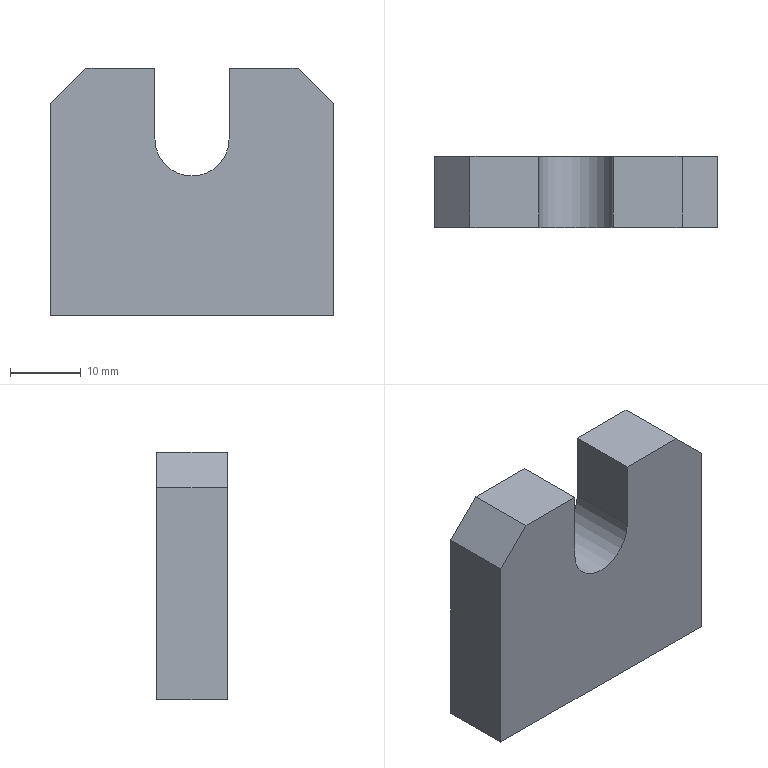Part | STEP file | PN_0038 | 1 solid | 20 faces | box 40 x 10 x 35 mm | volume 12065 mm3 | plane 11 | cylinder 5 | cone 4 | commonest cylinder face diameters 3.3 x4 10.5 x1
STEP:
#1=CARTESIAN_POINT('',(0.,0.,0.));
#2=DIRECTION('',(0.,0.,1.));
#3=DIRECTION('',(1.,0.,0.));
#4=AXIS2_PLACEMENT_3D('',#1,#2,#3);
#5=CARTESIAN_POINT('',(5.85,5.,-6.));
#6=VERTEX_POINT('',#5);
#7=CARTESIAN_POINT('',(5.85,5.,-17.5));
#8=VERTEX_POINT('',#7);
#9=CARTESIAN_POINT('',(5.85,5.,-17.5));
#10=DIRECTION('',(0.,0.,-1.));
#11=VECTOR('',#10,1.);
#12=LINE('',#9,#11);
#13=CARTESIAN_POINT('',(7.5,5.,-17.5));
#14=DIRECTION('',(0.,0.,-1.));
#15=DIRECTION('',(-1.,0.,0.));
#16=AXIS2_PLACEMENT_3D('',#13,#14,#15);
#17=CYLINDRICAL_SURFACE('',#16,1.65);
#18=CARTESIAN_POINT('',(6.283,0.));
#19=DIRECTION('',(0.,1.));
#20=VECTOR('',#19,1.);
#21=LINE('',#18,#20);
#22=(GEOMETRIC_REPRESENTATION_CONTEXT(2)PARAMETRIC_REPRESENTATION_CONTEXT()REPRESENTATION_CONTEXT('',''));
#23=DEFINITIONAL_REPRESENTATION('',(#21),#22);
#24=PCURVE('',#17,#23);
#25=CARTESIAN_POINT('',(7.5,5.,-17.5));
#26=DIRECTION('',(0.,0.,-1.));
#27=DIRECTION('',(-1.,0.,0.));
#28=AXIS2_PLACEMENT_3D('',#25,#26,#27);
#29=CYLINDRICAL_SURFACE('',#28,1.65);
#30=CARTESIAN_POINT('',(0.,0.));
#31=DIRECTION('',(0.,1.));
#32=VECTOR('',#31,1.);
#33=LINE('',#30,#32);
#34=(GEOMETRIC_REPRESENTATION_CONTEXT(2)PARAMETRIC_REPRESENTATION_CONTEXT()REPRESENTATION_CONTEXT('',''));
#35=DEFINITIONAL_REPRESENTATION('',(#33),#34);
#36=PCURVE('',#29,#35);
#37=SURFACE_CURVE('',#12,(#24,#36),.PCURVE_S1.);
#38=EDGE_CURVE('',#6,#8,#37,.T.);
#39=ORIENTED_EDGE('',*,*,#38,.T.);
#40=CARTESIAN_POINT('',(9.15,5.,-17.5));
#41=VERTEX_POINT('',#40);
#42=CARTESIAN_POINT('',(7.5,5.,-17.5));
#43=DIRECTION('',(0.,0.,-1.));
#44=DIRECTION('',(-1.,0.,0.));
#45=AXIS2_PLACEMENT_3D('',#42,#43,#44);
#46=CIRCLE('',#45,1.65);
#47=CARTESIAN_POINT('',(0.,0.));
#48=DIRECTION('',(1.,0.));
#49=VECTOR('',#48,1.);
#50=LINE('',#47,#49);
#51=(GEOMETRIC_REPRESENTATION_CONTEXT(2)PARAMETRIC_REPRESENTATION_CONTEXT()REPRESENTATION_CONTEXT('',''));
#52=DEFINITIONAL_REPRESENTATION('',(#50),#51);
#53=PCURVE('',#17,#52);
#54=CARTESIAN_POINT('',(-20.,10.,-17.5));
#55=DIRECTION('',(0.,0.,1.));
#56=DIRECTION('',(1.,0.,0.));
#57=AXIS2_PLACEMENT_3D('',#54,#55,#56);
#58=PLANE('',#57);
#59=CARTESIAN_POINT('',(25.85,-5.));
#60=CARTESIAN_POINT('',(25.85,-2.142));
#61=CARTESIAN_POINT('',(28.325,-3.571));
#62=CARTESIAN_POINT('',(30.8,-5.));
#63=CARTESIAN_POINT('',(28.325,-6.429));
#64=CARTESIAN_POINT('',(25.85,-7.858));
#65=CARTESIAN_POINT('',(25.85,-5.));
#66=(BOUNDED_CURVE()B_SPLINE_CURVE(2,(#59,#60,#61,#62,#63,#64,#65),.UNSPECIFIED.,.T.,.F.)B_SPLINE_CURVE_WITH_KNOTS((1,2,2,2,2,1),(-2.094,0.,2.094,4.189,6.283,8.378),.UNSPECIFIED.)CURVE()GEOMETRIC_REPRESENTATION_ITEM()RATIONAL_B_SPLINE_CURVE((1.,0.5,1.,0.5,1.,0.5,1.))REPRESENTATION_ITEM(''));
#67=(GEOMETRIC_REPRESENTATION_CONTEXT(2)PARAMETRIC_REPRESENTATION_CONTEXT()REPRESENTATION_CONTEXT('',''));
#68=DEFINITIONAL_REPRESENTATION('',(#66),#67);
#69=PCURVE('',#58,#68);
#70=SURFACE_CURVE('',#46,(#53,#69),.PCURVE_S1.);
#71=EDGE_CURVE('',#41,#8,#70,.T.);
#72=ORIENTED_EDGE('',*,*,#71,.F.);
#73=CARTESIAN_POINT('',(9.15,5.,-6.));
#74=VERTEX_POINT('',#73);
#75=CARTESIAN_POINT('',(9.15,5.,-17.5));
#76=DIRECTION('',(0.,0.,-1.));
#77=VECTOR('',#76,1.);
#78=LINE('',#75,#77);
#79=CARTESIAN_POINT('',(3.142,0.));
#80=DIRECTION('',(0.,1.));
#81=VECTOR('',#80,1.);
#82=LINE('',#79,#81);
#83=(GEOMETRIC_REPRESENTATION_CONTEXT(2)PARAMETRIC_REPRESENTATION_CONTEXT()REPRESENTATION_CONTEXT('',''));
#84=DEFINITIONAL_REPRESENTATION('',(#82),#83);
#85=PCURVE('',#17,#84);
#86=CARTESIAN_POINT('',(3.142,0.));
#87=DIRECTION('',(0.,1.));
#88=VECTOR('',#87,1.);
#89=LINE('',#86,#88);
#90=(GEOMETRIC_REPRESENTATION_CONTEXT(2)PARAMETRIC_REPRESENTATION_CONTEXT()REPRESENTATION_CONTEXT('',''));
#91=DEFINITIONAL_REPRESENTATION('',(#89),#90);
#92=PCURVE('',#29,#91);
#93=SURFACE_CURVE('',#78,(#85,#92),.PCURVE_S1.);
#94=EDGE_CURVE('',#74,#41,#93,.T.);
#95=ORIENTED_EDGE('',*,*,#94,.F.);
#96=CARTESIAN_POINT('',(7.5,5.,-6.));
#97=DIRECTION('',(0.,0.,-1.));
#98=DIRECTION('',(-1.,0.,0.));
#99=AXIS2_PLACEMENT_3D('',#96,#97,#98);
#100=CIRCLE('',#99,1.65);
#101=CARTESIAN_POINT('',(0.,-11.5));
#102=DIRECTION('',(1.,0.));
#103=VECTOR('',#102,1.);
#104=LINE('',#101,#103);
#105=(GEOMETRIC_REPRESENTATION_CONTEXT(2)PARAMETRIC_REPRESENTATION_CONTEXT()REPRESENTATION_CONTEXT('',''));
#106=DEFINITIONAL_REPRESENTATION('',(#104),#105);
#107=PCURVE('',#17,#106);
#108=CARTESIAN_POINT('',(7.5,5.,-6.));
#109=DIRECTION('',(0.,0.,-1.));
#110=DIRECTION('',(-1.,0.,0.));
#111=AXIS2_PLACEMENT_3D('',#108,#109,#110);
#112=CONICAL_SURFACE('',#111,1.65,1.03);
#113=CARTESIAN_POINT('',(0.,0.));
#114=DIRECTION('',(1.,0.));
#115=VECTOR('',#114,1.);
#116=LINE('',#113,#115);
#117=(GEOMETRIC_REPRESENTATION_CONTEXT(2)PARAMETRIC_REPRESENTATION_CONTEXT()REPRESENTATION_CONTEXT('',''));
#118=DEFINITIONAL_REPRESENTATION('',(#116),#117);
#119=PCURVE('',#112,#118);
#120=SURFACE_CURVE('',#100,(#107,#119),.PCURVE_S1.);
#121=EDGE_CURVE('',#74,#6,#120,.T.);
#122=ORIENTED_EDGE('',*,*,#121,.T.);
#123=EDGE_LOOP('',(#39,#72,#95,#122));
#124=FACE_BOUND('',#123,.F.);
#125=ADVANCED_FACE('',(#124),#17,.F.);
#126=ORIENTED_EDGE('',*,*,#121,.F.);
#127=CARTESIAN_POINT('',(7.5,5.,-5.009));
#128=VERTEX_POINT('',#127);
#129=CARTESIAN_POINT('',(9.15,5.,-6.));
#130=DIRECTION('',(0.8572,0.,-0.515));
#131=VECTOR('',#130,1.);
#132=LINE('',#129,#131);
#133=CARTESIAN_POINT('',(3.142,0.));
#134=DIRECTION('',(0.,1.));
#135=VECTOR('',#134,1.);
#136=LINE('',#133,#135);
#137=(GEOMETRIC_REPRESENTATION_CONTEXT(2)PARAMETRIC_REPRESENTATION_CONTEXT()REPRESENTATION_CONTEXT('',''));
#138=DEFINITIONAL_REPRESENTATION('',(#136),#137);
#139=PCURVE('',#112,#138);
#140=CARTESIAN_POINT('',(7.5,5.,-6.));
#141=DIRECTION('',(0.,0.,-1.));
#142=DIRECTION('',(-1.,0.,0.));
#143=AXIS2_PLACEMENT_3D('',#140,#141,#142);
#144=CONICAL_SURFACE('',#143,1.65,1.03);
#145=CARTESIAN_POINT('',(3.142,0.));
#146=DIRECTION('',(0.,1.));
#147=VECTOR('',#146,1.);
#148=LINE('',#145,#147);
#149=(GEOMETRIC_REPRESENTATION_CONTEXT(2)PARAMETRIC_REPRESENTATION_CONTEXT()REPRESENTATION_CONTEXT('',''));
#150=DEFINITIONAL_REPRESENTATION('',(#148),#149);
#151=PCURVE('',#144,#150);
#152=SURFACE_CURVE('',#132,(#139,#151),.PCURVE_S1.);
#153=EDGE_CURVE('',#128,#74,#152,.T.);
#154=ORIENTED_EDGE('',*,*,#153,.F.);
#155=CARTESIAN_POINT('',(5.85,5.,-6.));
#156=DIRECTION('',(-0.8572,0.,-0.515));
#157=VECTOR('',#156,1.);
#158=LINE('',#155,#157);
#159=CARTESIAN_POINT('',(6.283,0.));
#160=DIRECTION('',(0.,1.));
#161=VECTOR('',#160,1.);
#162=LINE('',#159,#161);
#163=(GEOMETRIC_REPRESENTATION_CONTEXT(2)PARAMETRIC_REPRESENTATION_CONTEXT()REPRESENTATION_CONTEXT('',''));
#164=DEFINITIONAL_REPRESENTATION('',(#162),#163);
#165=PCURVE('',#112,#164);
#166=CARTESIAN_POINT('',(0.,0.));
#167=DIRECTION('',(0.,1.));
#168=VECTOR('',#167,1.);
#169=LINE('',#166,#168);
#170=(GEOMETRIC_REPRESENTATION_CONTEXT(2)PARAMETRIC_REPRESENTATION_CONTEXT()REPRESENTATION_CONTEXT('',''));
#171=DEFINITIONAL_REPRESENTATION('',(#169),#170);
#172=PCURVE('',#144,#171);
#173=SURFACE_CURVE('',#158,(#165,#172),.PCURVE_S1.);
#174=EDGE_CURVE('',#128,#6,#173,.T.);
#175=ORIENTED_EDGE('',*,*,#174,.T.);
#176=EDGE_LOOP('',(#126,#154,#175));
#177=FACE_BOUND('',#176,.F.);
#178=ADVANCED_FACE('',(#177),#112,.F.);
#179=CARTESIAN_POINT('',(-9.15,5.,-6.));
#180=VERTEX_POINT('',#179);
#181=CARTESIAN_POINT('',(-9.15,5.,-17.5));
#182=VERTEX_POINT('',#181);
#183=CARTESIAN_POINT('',(-9.15,5.,-17.5));
#184=DIRECTION('',(0.,0.,-1.));
#185=VECTOR('',#184,1.);
#186=LINE('',#183,#185);
#187=CARTESIAN_POINT('',(-7.5,5.,-17.5));
#188=DIRECTION('',(0.,0.,-1.));
#189=DIRECTION('',(-1.,0.,0.));
#190=AXIS2_PLACEMENT_3D('',#187,#188,#189);
#191=CYLINDRICAL_SURFACE('',#190,1.65);
#192=CARTESIAN_POINT('',(6.283,0.));
#193=DIRECTION('',(0.,1.));
#194=VECTOR('',#193,1.);
#195=LINE('',#192,#194);
#196=(GEOMETRIC_REPRESENTATION_CONTEXT(2)PARAMETRIC_REPRESENTATION_CONTEXT()REPRESENTATION_CONTEXT('',''));
#197=DEFINITIONAL_REPRESENTATION('',(#195),#196);
#198=PCURVE('',#191,#197);
#199=CARTESIAN_POINT('',(-7.5,5.,-17.5));
#200=DIRECTION('',(0.,0.,-1.));
#201=DIRECTION('',(-1.,0.,0.));
#202=AXIS2_PLACEMENT_3D('',#199,#200,#201);
#203=CYLINDRICAL_SURFACE('',#202,1.65);
#204=CARTESIAN_POINT('',(0.,0.));
#205=DIRECTION('',(0.,1.));
#206=VECTOR('',#205,1.);
#207=LINE('',#204,#206);
#208=(GEOMETRIC_REPRESENTATION_CONTEXT(2)PARAMETRIC_REPRESENTATION_CONTEXT()REPRESENTATION_CONTEXT('',''));
#209=DEFINITIONAL_REPRESENTATION('',(#207),#208);
#210=PCURVE('',#203,#209);
#211=SURFACE_CURVE('',#186,(#198,#210),.PCURVE_S1.);
#212=EDGE_CURVE('',#180,#182,#211,.T.);
#213=ORIENTED_EDGE('',*,*,#212,.T.);
#214=CARTESIAN_POINT('',(-5.85,5.,-17.5));
#215=VERTEX_POINT('',#214);
#216=CARTESIAN_POINT('',(-7.5,5.,-17.5));
#217=DIRECTION('',(0.,0.,-1.));
#218=DIRECTION('',(-1.,0.,0.));
#219=AXIS2_PLACEMENT_3D('',#216,#217,#218);
#220=CIRCLE('',#219,1.65);
#221=CARTESIAN_POINT('',(0.,0.));
#222=DIRECTION('',(1.,0.));
#223=VECTOR('',#222,1.);
#224=LINE('',#221,#223);
#225=(GEOMETRIC_REPRESENTATION_CONTEXT(2)PARAMETRIC_REPRESENTATION_CONTEXT()REPRESENTATION_CONTEXT('',''));
#226=DEFINITIONAL_REPRESENTATION('',(#224),#225);
#227=PCURVE('',#191,#226);
#228=CARTESIAN_POINT('',(10.85,-5.));
#229=CARTESIAN_POINT('',(10.85,-2.142));
#230=CARTESIAN_POINT('',(13.325,-3.571));
#231=CARTESIAN_POINT('',(15.8,-5.));
#232=CARTESIAN_POINT('',(13.325,-6.429));
#233=CARTESIAN_POINT('',(10.85,-7.858));
#234=CARTESIAN_POINT('',(10.85,-5.));
#235=(BOUNDED_CURVE()B_SPLINE_CURVE(2,(#228,#229,#230,#231,#232,#233,#234),.UNSPECIFIED.,.T.,.F.)B_SPLINE_CURVE_WITH_KNOTS((1,2,2,2,2,1),(-2.094,0.,2.094,4.189,6.283,8.378),.UNSPECIFIED.)CURVE()GEOMETRIC_REPRESENTATION_ITEM()RATIONAL_B_SPLINE_CURVE((1.,0.5,1.,0.5,1.,0.5,1.))REPRESENTATION_ITEM(''));
#236=(GEOMETRIC_REPRESENTATION_CONTEXT(2)PARAMETRIC_REPRESENTATION_CONTEXT()REPRESENTATION_CONTEXT('',''));
#237=DEFINITIONAL_REPRESENTATION('',(#235),#236);
#238=PCURVE('',#58,#237);
#239=SURFACE_CURVE('',#220,(#227,#238),.PCURVE_S1.);
#240=EDGE_CURVE('',#215,#182,#239,.T.);
#241=ORIENTED_EDGE('',*,*,#240,.F.);
#242=CARTESIAN_POINT('',(-5.85,5.,-6.));
#243=VERTEX_POINT('',#242);
#244=CARTESIAN_POINT('',(-5.85,5.,-17.5));
#245=DIRECTION('',(0.,0.,-1.));
#246=VECTOR('',#245,1.);
#247=LINE('',#244,#246);
#248=CARTESIAN_POINT('',(3.142,0.));
#249=DIRECTION('',(0.,1.));
#250=VECTOR('',#249,1.);
#251=LINE('',#248,#250);
#252=(GEOMETRIC_REPRESENTATION_CONTEXT(2)PARAMETRIC_REPRESENTATION_CONTEXT()REPRESENTATION_CONTEXT('',''));
#253=DEFINITIONAL_REPRESENTATION('',(#251),#252);
#254=PCURVE('',#191,#253);
#255=CARTESIAN_POINT('',(3.142,0.));
#256=DIRECTION('',(0.,1.));
#257=VECTOR('',#256,1.);
#258=LINE('',#255,#257);
#259=(GEOMETRIC_REPRESENTATION_CONTEXT(2)PARAMETRIC_REPRESENTATION_CONTEXT()REPRESENTATION_CONTEXT('',''));
#260=DEFINITIONAL_REPRESENTATION('',(#258),#259);
#261=PCURVE('',#203,#260);
#262=SURFACE_CURVE('',#247,(#254,#261),.PCURVE_S1.);
#263=EDGE_CURVE('',#243,#215,#262,.T.);
#264=ORIENTED_EDGE('',*,*,#263,.F.);
#265=CARTESIAN_POINT('',(-7.5,5.,-6.));
#266=DIRECTION('',(0.,0.,-1.));
#267=DIRECTION('',(-1.,0.,0.));
#268=AXIS2_PLACEMENT_3D('',#265,#266,#267);
#269=CIRCLE('',#268,1.65);
#270=CARTESIAN_POINT('',(0.,-11.5));
#271=DIRECTION('',(1.,0.));
#272=VECTOR('',#271,1.);
#273=LINE('',#270,#272);
#274=(GEOMETRIC_REPRESENTATION_CONTEXT(2)PARAMETRIC_REPRESENTATION_CONTEXT()REPRESENTATION_CONTEXT('',''));
#275=DEFINITIONAL_REPRESENTATION('',(#273),#274);
#276=PCURVE('',#191,#275);
#277=CARTESIAN_POINT('',(-7.5,5.,-6.));
#278=DIRECTION('',(0.,0.,-1.));
#279=DIRECTION('',(-1.,0.,0.));
#280=AXIS2_PLACEMENT_3D('',#277,#278,#279);
#281=CONICAL_SURFACE('',#280,1.65,1.03);
#282=CARTESIAN_POINT('',(0.,0.));
#283=DIRECTION('',(1.,0.));
#284=VECTOR('',#283,1.);
#285=LINE('',#282,#284);
#286=(GEOMETRIC_REPRESENTATION_CONTEXT(2)PARAMETRIC_REPRESENTATION_CONTEXT()REPRESENTATION_CONTEXT('',''));
#287=DEFINITIONAL_REPRESENTATION('',(#285),#286);
#288=PCURVE('',#281,#287);
#289=SURFACE_CURVE('',#269,(#276,#288),.PCURVE_S1.);
#290=EDGE_CURVE('',#243,#180,#289,.T.);
#291=ORIENTED_EDGE('',*,*,#290,.T.);
#292=EDGE_LOOP('',(#213,#241,#264,#291));
#293=FACE_BOUND('',#292,.F.);
#294=ADVANCED_FACE('',(#293),#191,.F.);
#295=ORIENTED_EDGE('',*,*,#290,.F.);
#296=CARTESIAN_POINT('',(-7.5,5.,-5.009));
#297=VERTEX_POINT('',#296);
#298=CARTESIAN_POINT('',(-5.85,5.,-6.));
#299=DIRECTION('',(0.8572,0.,-0.515));
#300=VECTOR('',#299,1.);
#301=LINE('',#298,#300);
#302=CARTESIAN_POINT('',(3.142,0.));
#303=DIRECTION('',(0.,1.));
#304=VECTOR('',#303,1.);
#305=LINE('',#302,#304);
#306=(GEOMETRIC_REPRESENTATION_CONTEXT(2)PARAMETRIC_REPRESENTATION_CONTEXT()REPRESENTATION_CONTEXT('',''));
#307=DEFINITIONAL_REPRESENTATION('',(#305),#306);
#308=PCURVE('',#281,#307);
#309=CARTESIAN_POINT('',(-7.5,5.,-6.));
#310=DIRECTION('',(0.,0.,-1.));
#311=DIRECTION('',(-1.,0.,0.));
#312=AXIS2_PLACEMENT_3D('',#309,#310,#311);
#313=CONICAL_SURFACE('',#312,1.65,1.03);
#314=CARTESIAN_POINT('',(3.142,0.));
#315=DIRECTION('',(0.,1.));
#316=VECTOR('',#315,1.);
#317=LINE('',#314,#316);
#318=(GEOMETRIC_REPRESENTATION_CONTEXT(2)PARAMETRIC_REPRESENTATION_CONTEXT()REPRESENTATION_CONTEXT('',''));
#319=DEFINITIONAL_REPRESENTATION('',(#317),#318);
#320=PCURVE('',#313,#319);
#321=SURFACE_CURVE('',#301,(#308,#320),.PCURVE_S1.);
#322=EDGE_CURVE('',#297,#243,#321,.T.);
#323=ORIENTED_EDGE('',*,*,#322,.F.);
#324=CARTESIAN_POINT('',(-9.15,5.,-6.));
#325=DIRECTION('',(-0.8572,0.,-0.515));
#326=VECTOR('',#325,1.);
#327=LINE('',#324,#326);
#328=CARTESIAN_POINT('',(6.283,0.));
#329=DIRECTION('',(0.,1.));
#330=VECTOR('',#329,1.);
#331=LINE('',#328,#330);
#332=(GEOMETRIC_REPRESENTATION_CONTEXT(2)PARAMETRIC_REPRESENTATION_CONTEXT()REPRESENTATION_CONTEXT('',''));
#333=DEFINITIONAL_REPRESENTATION('',(#331),#332);
#334=PCURVE('',#281,#333);
#335=CARTESIAN_POINT('',(0.,0.));
#336=DIRECTION('',(0.,1.));
#337=VECTOR('',#336,1.);
#338=LINE('',#335,#337);
#339=(GEOMETRIC_REPRESENTATION_CONTEXT(2)PARAMETRIC_REPRESENTATION_CONTEXT()REPRESENTATION_CONTEXT('',''));
#340=DEFINITIONAL_REPRESENTATION('',(#338),#339);
#341=PCURVE('',#313,#340);
#342=SURFACE_CURVE('',#327,(#334,#341),.PCURVE_S1.);
#343=EDGE_CURVE('',#297,#180,#342,.T.);
#344=ORIENTED_EDGE('',*,*,#343,.T.);
#345=EDGE_LOOP('',(#295,#323,#344));
#346=FACE_BOUND('',#345,.F.);
#347=ADVANCED_FACE('',(#346),#281,.F.);
#348=CARTESIAN_POINT('',(5.25,10.,17.5));
#349=VERTEX_POINT('',#348);
#350=CARTESIAN_POINT('',(15.,10.,17.5));
#351=VERTEX_POINT('',#350);
#352=CARTESIAN_POINT('',(-20.,10.,17.5));
#353=DIRECTION('',(1.,0.,0.));
#354=VECTOR('',#353,1.);
#355=LINE('',#352,#354);
#356=CARTESIAN_POINT('',(-20.,10.,17.5));
#357=DIRECTION('',(0.,0.,-1.));
#358=DIRECTION('',(-1.,0.,0.));
#359=AXIS2_PLACEMENT_3D('',#356,#357,#358);
#360=PLANE('',#359);
#361=CARTESIAN_POINT('',(0.,0.));
#362=DIRECTION('',(-1.,0.));
#363=VECTOR('',#362,1.);
#364=LINE('',#361,#363);
#365=(GEOMETRIC_REPRESENTATION_CONTEXT(2)PARAMETRIC_REPRESENTATION_CONTEXT()REPRESENTATION_CONTEXT('',''));
#366=DEFINITIONAL_REPRESENTATION('',(#364),#365);
#367=PCURVE('',#360,#366);
#368=CARTESIAN_POINT('',(0.,10.,0.));
#369=DIRECTION('',(0.,1.,0.));
#370=DIRECTION('',(0.,0.,1.));
#371=AXIS2_PLACEMENT_3D('',#368,#369,#370);
#372=PLANE('',#371);
#373=CARTESIAN_POINT('',(17.5,-20.));
#374=DIRECTION('',(0.,1.));
#375=VECTOR('',#374,1.);
#376=LINE('',#373,#375);
#377=(GEOMETRIC_REPRESENTATION_CONTEXT(2)PARAMETRIC_REPRESENTATION_CONTEXT()REPRESENTATION_CONTEXT('',''));
#378=DEFINITIONAL_REPRESENTATION('',(#376),#377);
#379=PCURVE('',#372,#378);
#380=SURFACE_CURVE('',#355,(#367,#379),.PCURVE_S1.);
#381=EDGE_CURVE('',#349,#351,#380,.T.);
#382=ORIENTED_EDGE('',*,*,#381,.F.);
#383=CARTESIAN_POINT('',(5.25,0.,17.5));
#384=VERTEX_POINT('',#383);
#385=CARTESIAN_POINT('',(5.25,0.,17.5));
#386=DIRECTION('',(0.,1.,0.));
#387=VECTOR('',#386,1.);
#388=LINE('',#385,#387);
#389=CARTESIAN_POINT('',(-25.25,-10.));
#390=DIRECTION('',(0.,1.));
#391=VECTOR('',#390,1.);
#392=LINE('',#389,#391);
#393=(GEOMETRIC_REPRESENTATION_CONTEXT(2)PARAMETRIC_REPRESENTATION_CONTEXT()REPRESENTATION_CONTEXT('',''));
#394=DEFINITIONAL_REPRESENTATION('',(#392),#393);
#395=PCURVE('',#360,#394);
#396=CARTESIAN_POINT('',(5.25,0.,7.5));
#397=DIRECTION('',(1.,0.,0.));
#398=DIRECTION('',(0.,0.,-1.));
#399=AXIS2_PLACEMENT_3D('',#396,#397,#398);
#400=PLANE('',#399);
#401=CARTESIAN_POINT('',(-10.,0.));
#402=DIRECTION('',(0.,1.));
#403=VECTOR('',#402,1.);
#404=LINE('',#401,#403);
#405=(GEOMETRIC_REPRESENTATION_CONTEXT(2)PARAMETRIC_REPRESENTATION_CONTEXT()REPRESENTATION_CONTEXT('',''));
#406=DEFINITIONAL_REPRESENTATION('',(#404),#405);
#407=PCURVE('',#400,#406);
#408=SURFACE_CURVE('',#388,(#395,#407),.PCURVE_S1.);
#409=EDGE_CURVE('',#384,#349,#408,.T.);
#410=ORIENTED_EDGE('',*,*,#409,.F.);
#411=CARTESIAN_POINT('',(15.,0.,17.5));
#412=VERTEX_POINT('',#411);
#413=CARTESIAN_POINT('',(-20.,0.,17.5));
#414=DIRECTION('',(1.,0.,0.));
#415=VECTOR('',#414,1.);
#416=LINE('',#413,#415);
#417=CARTESIAN_POINT('',(0.,-10.));
#418=DIRECTION('',(-1.,0.));
#419=VECTOR('',#418,1.);
#420=LINE('',#417,#419);
#421=(GEOMETRIC_REPRESENTATION_CONTEXT(2)PARAMETRIC_REPRESENTATION_CONTEXT()REPRESENTATION_CONTEXT('',''));
#422=DEFINITIONAL_REPRESENTATION('',(#420),#421);
#423=PCURVE('',#360,#422);
#424=CARTESIAN_POINT('',(0.,0.,0.));
#425=DIRECTION('',(0.,1.,0.));
#426=DIRECTION('',(0.,0.,1.));
#427=AXIS2_PLACEMENT_3D('',#424,#425,#426);
#428=PLANE('',#427);
#429=CARTESIAN_POINT('',(17.5,-20.));
#430=DIRECTION('',(0.,1.));
#431=VECTOR('',#430,1.);
#432=LINE('',#429,#431);
#433=(GEOMETRIC_REPRESENTATION_CONTEXT(2)PARAMETRIC_REPRESENTATION_CONTEXT()REPRESENTATION_CONTEXT('',''));
#434=DEFINITIONAL_REPRESENTATION('',(#432),#433);
#435=PCURVE('',#428,#434);
#436=SURFACE_CURVE('',#416,(#423,#435),.PCURVE_S1.);
#437=EDGE_CURVE('',#384,#412,#436,.T.);
#438=ORIENTED_EDGE('',*,*,#437,.T.);
#439=CARTESIAN_POINT('',(15.,10.,17.5));
#440=DIRECTION('',(0.,1.,0.));
#441=VECTOR('',#440,1.);
#442=LINE('',#439,#441);
#443=CARTESIAN_POINT('',(-35.,0.));
#444=DIRECTION('',(0.,1.));
#445=VECTOR('',#444,1.);
#446=LINE('',#443,#445);
#447=(GEOMETRIC_REPRESENTATION_CONTEXT(2)PARAMETRIC_REPRESENTATION_CONTEXT()REPRESENTATION_CONTEXT('',''));
#448=DEFINITIONAL_REPRESENTATION('',(#446),#447);
#449=PCURVE('',#360,#448);
#450=CARTESIAN_POINT('',(20.,10.,12.5));
#451=DIRECTION('',(-0.7071,0.,-0.7071));
#452=DIRECTION('',(0.,-1.,0.));
#453=AXIS2_PLACEMENT_3D('',#450,#451,#452);
#454=PLANE('',#453);
#455=CARTESIAN_POINT('',(0.,7.071));
#456=DIRECTION('',(-1.,0.));
#457=VECTOR('',#456,1.);
#458=LINE('',#455,#457);
#459=(GEOMETRIC_REPRESENTATION_CONTEXT(2)PARAMETRIC_REPRESENTATION_CONTEXT()REPRESENTATION_CONTEXT('',''));
#460=DEFINITIONAL_REPRESENTATION('',(#458),#459);
#461=PCURVE('',#454,#460);
#462=SURFACE_CURVE('',#442,(#449,#461),.PCURVE_S1.);
#463=EDGE_CURVE('',#412,#351,#462,.T.);
#464=ORIENTED_EDGE('',*,*,#463,.T.);
#465=EDGE_LOOP('',(#382,#410,#438,#464));
#466=FACE_BOUND('',#465,.T.);
#467=ADVANCED_FACE('',(#466),#360,.F.);
#468=CARTESIAN_POINT('',(20.,10.,12.5));
#469=VERTEX_POINT('',#468);
#470=CARTESIAN_POINT('',(20.,10.,-17.5));
#471=VERTEX_POINT('',#470);
#472=CARTESIAN_POINT('',(20.,10.,-17.5));
#473=DIRECTION('',(0.,0.,-1.));
#474=VECTOR('',#473,1.);
#475=LINE('',#472,#474);
#476=CARTESIAN_POINT('',(20.,10.,-17.5));
#477=DIRECTION('',(-1.,0.,0.));
#478=DIRECTION('',(0.,0.,1.));
#479=AXIS2_PLACEMENT_3D('',#476,#477,#478);
#480=PLANE('',#479);
#481=CARTESIAN_POINT('',(0.,0.));
#482=DIRECTION('',(-1.,0.));
#483=VECTOR('',#482,1.);
#484=LINE('',#481,#483);
#485=(GEOMETRIC_REPRESENTATION_CONTEXT(2)PARAMETRIC_REPRESENTATION_CONTEXT()REPRESENTATION_CONTEXT('',''));
#486=DEFINITIONAL_REPRESENTATION('',(#484),#485);
#487=PCURVE('',#480,#486);
#488=CARTESIAN_POINT('',(-17.5,20.));
#489=DIRECTION('',(-1.,0.));
#490=VECTOR('',#489,1.);
#491=LINE('',#488,#490);
#492=(GEOMETRIC_REPRESENTATION_CONTEXT(2)PARAMETRIC_REPRESENTATION_CONTEXT()REPRESENTATION_CONTEXT('',''));
#493=DEFINITIONAL_REPRESENTATION('',(#491),#492);
#494=PCURVE('',#372,#493);
#495=SURFACE_CURVE('',#475,(#487,#494),.PCURVE_S1.);
#496=EDGE_CURVE('',#469,#471,#495,.T.);
#497=ORIENTED_EDGE('',*,*,#496,.F.);
#498=CARTESIAN_POINT('',(20.,0.,12.5));
#499=VERTEX_POINT('',#498);
#500=CARTESIAN_POINT('',(20.,10.,12.5));
#501=DIRECTION('',(0.,-1.,0.));
#502=VECTOR('',#501,1.);
#503=LINE('',#500,#502);
#504=CARTESIAN_POINT('',(30.,0.));
#505=DIRECTION('',(0.,-1.));
#506=VECTOR('',#505,1.);
#507=LINE('',#504,#506);
#508=(GEOMETRIC_REPRESENTATION_CONTEXT(2)PARAMETRIC_REPRESENTATION_CONTEXT()REPRESENTATION_CONTEXT('',''));
#509=DEFINITIONAL_REPRESENTATION('',(#507),#508);
#510=PCURVE('',#480,#509);
#511=CARTESIAN_POINT('',(0.,0.));
#512=DIRECTION('',(1.,0.));
#513=VECTOR('',#512,1.);
#514=LINE('',#511,#513);
#515=(GEOMETRIC_REPRESENTATION_CONTEXT(2)PARAMETRIC_REPRESENTATION_CONTEXT()REPRESENTATION_CONTEXT('',''));
#516=DEFINITIONAL_REPRESENTATION('',(#514),#515);
#517=PCURVE('',#454,#516);
#518=SURFACE_CURVE('',#503,(#510,#517),.PCURVE_S1.);
#519=EDGE_CURVE('',#469,#499,#518,.T.);
#520=ORIENTED_EDGE('',*,*,#519,.T.);
#521=CARTESIAN_POINT('',(20.,0.,-17.5));
#522=VERTEX_POINT('',#521);
#523=CARTESIAN_POINT('',(20.,0.,-17.5));
#524=DIRECTION('',(0.,0.,-1.));
#525=VECTOR('',#524,1.);
#526=LINE('',#523,#525);
#527=CARTESIAN_POINT('',(0.,-10.));
#528=DIRECTION('',(-1.,0.));
#529=VECTOR('',#528,1.);
#530=LINE('',#527,#529);
#531=(GEOMETRIC_REPRESENTATION_CONTEXT(2)PARAMETRIC_REPRESENTATION_CONTEXT()REPRESENTATION_CONTEXT('',''));
#532=DEFINITIONAL_REPRESENTATION('',(#530),#531);
#533=PCURVE('',#480,#532);
#534=CARTESIAN_POINT('',(-17.5,20.));
#535=DIRECTION('',(-1.,0.));
#536=VECTOR('',#535,1.);
#537=LINE('',#534,#536);
#538=(GEOMETRIC_REPRESENTATION_CONTEXT(2)PARAMETRIC_REPRESENTATION_CONTEXT()REPRESENTATION_CONTEXT('',''));
#539=DEFINITIONAL_REPRESENTATION('',(#537),#538);
#540=PCURVE('',#428,#539);
#541=SURFACE_CURVE('',#526,(#533,#540),.PCURVE_S1.);
#542=EDGE_CURVE('',#499,#522,#541,.T.);
#543=ORIENTED_EDGE('',*,*,#542,.T.);
#544=CARTESIAN_POINT('',(20.,10.,-17.5));
#545=DIRECTION('',(0.,-1.,0.));
#546=VECTOR('',#545,1.);
#547=LINE('',#544,#546);
#548=CARTESIAN_POINT('',(0.,0.));
#549=DIRECTION('',(0.,-1.));
#550=VECTOR('',#549,1.);
#551=LINE('',#548,#550);
#552=(GEOMETRIC_REPRESENTATION_CONTEXT(2)PARAMETRIC_REPRESENTATION_CONTEXT()REPRESENTATION_CONTEXT('',''));
#553=DEFINITIONAL_REPRESENTATION('',(#551),#552);
#554=PCURVE('',#480,#553);
#555=CARTESIAN_POINT('',(40.,0.));
#556=DIRECTION('',(0.,-1.));
#557=VECTOR('',#556,1.);
#558=LINE('',#555,#557);
#559=(GEOMETRIC_REPRESENTATION_CONTEXT(2)PARAMETRIC_REPRESENTATION_CONTEXT()REPRESENTATION_CONTEXT('',''));
#560=DEFINITIONAL_REPRESENTATION('',(#558),#559);
#561=PCURVE('',#58,#560);
#562=SURFACE_CURVE('',#547,(#554,#561),.PCURVE_S1.);
#563=EDGE_CURVE('',#471,#522,#562,.T.);
#564=ORIENTED_EDGE('',*,*,#563,.F.);
#565=EDGE_LOOP('',(#497,#520,#543,#564));
#566=FACE_BOUND('',#565,.T.);
#567=ADVANCED_FACE('',(#566),#480,.F.);
#568=CARTESIAN_POINT('',(7.5,5.,-17.5));
#569=DIRECTION('',(0.,0.,-1.));
#570=DIRECTION('',(-1.,0.,0.));
#571=AXIS2_PLACEMENT_3D('',#568,#569,#570);
#572=CIRCLE('',#571,1.65);
#573=CARTESIAN_POINT('',(25.85,-5.));
#574=CARTESIAN_POINT('',(25.85,-2.142));
#575=CARTESIAN_POINT('',(28.325,-3.571));
#576=CARTESIAN_POINT('',(30.8,-5.));
#577=CARTESIAN_POINT('',(28.325,-6.429));
#578=CARTESIAN_POINT('',(25.85,-7.858));
#579=CARTESIAN_POINT('',(25.85,-5.));
#580=(BOUNDED_CURVE()B_SPLINE_CURVE(2,(#573,#574,#575,#576,#577,#578,#579),.UNSPECIFIED.,.T.,.F.)B_SPLINE_CURVE_WITH_KNOTS((1,2,2,2,2,1),(-2.094,0.,2.094,4.189,6.283,8.378),.UNSPECIFIED.)CURVE()GEOMETRIC_REPRESENTATION_ITEM()RATIONAL_B_SPLINE_CURVE((1.,0.5,1.,0.5,1.,0.5,1.))REPRESENTATION_ITEM(''));
#581=(GEOMETRIC_REPRESENTATION_CONTEXT(2)PARAMETRIC_REPRESENTATION_CONTEXT()REPRESENTATION_CONTEXT('',''));
#582=DEFINITIONAL_REPRESENTATION('',(#580),#581);
#583=PCURVE('',#58,#582);
#584=CARTESIAN_POINT('',(0.,0.));
#585=DIRECTION('',(1.,0.));
#586=VECTOR('',#585,1.);
#587=LINE('',#584,#586);
#588=(GEOMETRIC_REPRESENTATION_CONTEXT(2)PARAMETRIC_REPRESENTATION_CONTEXT()REPRESENTATION_CONTEXT('',''));
#589=DEFINITIONAL_REPRESENTATION('',(#587),#588);
#590=PCURVE('',#29,#589);
#591=SURFACE_CURVE('',#572,(#583,#590),.PCURVE_S1.);
#592=EDGE_CURVE('',#8,#41,#591,.T.);
#593=ORIENTED_EDGE('',*,*,#592,.F.);
#594=ORIENTED_EDGE('',*,*,#71,.F.);
#595=EDGE_LOOP('',(#593,#594));
#596=FACE_BOUND('',#595,.T.);
#597=CARTESIAN_POINT('',(-7.5,5.,-17.5));
#598=DIRECTION('',(0.,0.,-1.));
#599=DIRECTION('',(-1.,0.,0.));
#600=AXIS2_PLACEMENT_3D('',#597,#598,#599);
#601=CIRCLE('',#600,1.65);
#602=CARTESIAN_POINT('',(10.85,-5.));
#603=CARTESIAN_POINT('',(10.85,-2.142));
#604=CARTESIAN_POINT('',(13.325,-3.571));
#605=CARTESIAN_POINT('',(15.8,-5.));
#606=CARTESIAN_POINT('',(13.325,-6.429));
#607=CARTESIAN_POINT('',(10.85,-7.858));
#608=CARTESIAN_POINT('',(10.85,-5.));
#609=(BOUNDED_CURVE()B_SPLINE_CURVE(2,(#602,#603,#604,#605,#606,#607,#608),.UNSPECIFIED.,.T.,.F.)B_SPLINE_CURVE_WITH_KNOTS((1,2,2,2,2,1),(-2.094,0.,2.094,4.189,6.283,8.378),.UNSPECIFIED.)CURVE()GEOMETRIC_REPRESENTATION_ITEM()RATIONAL_B_SPLINE_CURVE((1.,0.5,1.,0.5,1.,0.5,1.))REPRESENTATION_ITEM(''));
#610=(GEOMETRIC_REPRESENTATION_CONTEXT(2)PARAMETRIC_REPRESENTATION_CONTEXT()REPRESENTATION_CONTEXT('',''));
#611=DEFINITIONAL_REPRESENTATION('',(#609),#610);
#612=PCURVE('',#58,#611);
#613=CARTESIAN_POINT('',(0.,0.));
#614=DIRECTION('',(1.,0.));
#615=VECTOR('',#614,1.);
#616=LINE('',#613,#615);
#617=(GEOMETRIC_REPRESENTATION_CONTEXT(2)PARAMETRIC_REPRESENTATION_CONTEXT()REPRESENTATION_CONTEXT('',''));
#618=DEFINITIONAL_REPRESENTATION('',(#616),#617);
#619=PCURVE('',#203,#618);
#620=SURFACE_CURVE('',#601,(#612,#619),.PCURVE_S1.);
#621=EDGE_CURVE('',#182,#215,#620,.T.);
#622=ORIENTED_EDGE('',*,*,#621,.F.);
#623=ORIENTED_EDGE('',*,*,#240,.F.);
#624=EDGE_LOOP('',(#622,#623));
#625=FACE_BOUND('',#624,.T.);
#626=CARTESIAN_POINT('',(-20.,0.,-17.5));
#627=VERTEX_POINT('',#626);
#628=CARTESIAN_POINT('',(-20.,0.,-17.5));
#629=DIRECTION('',(-1.,0.,0.));
#630=VECTOR('',#629,1.);
#631=LINE('',#628,#630);
#632=CARTESIAN_POINT('',(0.,-10.));
#633=DIRECTION('',(-1.,0.));
#634=VECTOR('',#633,1.);
#635=LINE('',#632,#634);
#636=(GEOMETRIC_REPRESENTATION_CONTEXT(2)PARAMETRIC_REPRESENTATION_CONTEXT()REPRESENTATION_CONTEXT('',''));
#637=DEFINITIONAL_REPRESENTATION('',(#635),#636);
#638=PCURVE('',#58,#637);
#639=CARTESIAN_POINT('',(-17.5,-20.));
#640=DIRECTION('',(0.,-1.));
#641=VECTOR('',#640,1.);
#642=LINE('',#639,#641);
#643=(GEOMETRIC_REPRESENTATION_CONTEXT(2)PARAMETRIC_REPRESENTATION_CONTEXT()REPRESENTATION_CONTEXT('',''));
#644=DEFINITIONAL_REPRESENTATION('',(#642),#643);
#645=PCURVE('',#428,#644);
#646=SURFACE_CURVE('',#631,(#638,#645),.PCURVE_S1.);
#647=EDGE_CURVE('',#522,#627,#646,.T.);
#648=ORIENTED_EDGE('',*,*,#647,.T.);
#649=CARTESIAN_POINT('',(-20.,10.,-17.5));
#650=VERTEX_POINT('',#649);
#651=CARTESIAN_POINT('',(-20.,10.,-17.5));
#652=DIRECTION('',(0.,-1.,0.));
#653=VECTOR('',#652,1.);
#654=LINE('',#651,#653);
#655=CARTESIAN_POINT('',(0.,0.));
#656=DIRECTION('',(0.,-1.));
#657=VECTOR('',#656,1.);
#658=LINE('',#655,#657);
#659=(GEOMETRIC_REPRESENTATION_CONTEXT(2)PARAMETRIC_REPRESENTATION_CONTEXT()REPRESENTATION_CONTEXT('',''));
#660=DEFINITIONAL_REPRESENTATION('',(#658),#659);
#661=PCURVE('',#58,#660);
#662=CARTESIAN_POINT('',(-20.,10.,-17.5));
#663=DIRECTION('',(1.,0.,0.));
#664=DIRECTION('',(0.,0.,-1.));
#665=AXIS2_PLACEMENT_3D('',#662,#663,#664);
#666=PLANE('',#665);
#667=CARTESIAN_POINT('',(0.,0.));
#668=DIRECTION('',(0.,-1.));
#669=VECTOR('',#668,1.);
#670=LINE('',#667,#669);
#671=(GEOMETRIC_REPRESENTATION_CONTEXT(2)PARAMETRIC_REPRESENTATION_CONTEXT()REPRESENTATION_CONTEXT('',''));
#672=DEFINITIONAL_REPRESENTATION('',(#670),#671);
#673=PCURVE('',#666,#672);
#674=SURFACE_CURVE('',#654,(#661,#673),.PCURVE_S1.);
#675=EDGE_CURVE('',#650,#627,#674,.T.);
#676=ORIENTED_EDGE('',*,*,#675,.F.);
#677=CARTESIAN_POINT('',(-20.,10.,-17.5));
#678=DIRECTION('',(-1.,0.,0.));
#679=VECTOR('',#678,1.);
#680=LINE('',#677,#679);
#681=CARTESIAN_POINT('',(0.,0.));
#682=DIRECTION('',(-1.,0.));
#683=VECTOR('',#682,1.);
#684=LINE('',#681,#683);
#685=(GEOMETRIC_REPRESENTATION_CONTEXT(2)PARAMETRIC_REPRESENTATION_CONTEXT()REPRESENTATION_CONTEXT('',''));
#686=DEFINITIONAL_REPRESENTATION('',(#684),#685);
#687=PCURVE('',#58,#686);
#688=CARTESIAN_POINT('',(-17.5,-20.));
#689=DIRECTION('',(0.,-1.));
#690=VECTOR('',#689,1.);
#691=LINE('',#688,#690);
#692=(GEOMETRIC_REPRESENTATION_CONTEXT(2)PARAMETRIC_REPRESENTATION_CONTEXT()REPRESENTATION_CONTEXT('',''));
#693=DEFINITIONAL_REPRESENTATION('',(#691),#692);
#694=PCURVE('',#372,#693);
#695=SURFACE_CURVE('',#680,(#687,#694),.PCURVE_S1.);
#696=EDGE_CURVE('',#471,#650,#695,.T.);
#697=ORIENTED_EDGE('',*,*,#696,.F.);
#698=ORIENTED_EDGE('',*,*,#563,.T.);
#699=EDGE_LOOP('',(#648,#676,#697,#698));
#700=FACE_BOUND('',#699,.T.);
#701=ADVANCED_FACE('',(#596,#625,#700),#58,.F.);
#702=CARTESIAN_POINT('',(-20.,0.,12.5));
#703=VERTEX_POINT('',#702);
#704=CARTESIAN_POINT('',(-20.,0.,-17.5));
#705=DIRECTION('',(0.,0.,1.));
#706=VECTOR('',#705,1.);
#707=LINE('',#704,#706);
#708=CARTESIAN_POINT('',(0.,-10.));
#709=DIRECTION('',(-1.,0.));
#710=VECTOR('',#709,1.);
#711=LINE('',#708,#710);
#712=(GEOMETRIC_REPRESENTATION_CONTEXT(2)PARAMETRIC_REPRESENTATION_CONTEXT()REPRESENTATION_CONTEXT('',''));
#713=DEFINITIONAL_REPRESENTATION('',(#711),#712);
#714=PCURVE('',#666,#713);
#715=CARTESIAN_POINT('',(-17.5,-20.));
#716=DIRECTION('',(1.,0.));
#717=VECTOR('',#716,1.);
#718=LINE('',#715,#717);
#719=(GEOMETRIC_REPRESENTATION_CONTEXT(2)PARAMETRIC_REPRESENTATION_CONTEXT()REPRESENTATION_CONTEXT('',''));
#720=DEFINITIONAL_REPRESENTATION('',(#718),#719);
#721=PCURVE('',#428,#720);
#722=SURFACE_CURVE('',#707,(#714,#721),.PCURVE_S1.);
#723=EDGE_CURVE('',#627,#703,#722,.T.);
#724=ORIENTED_EDGE('',*,*,#723,.T.);
#725=CARTESIAN_POINT('',(-20.,10.,12.5));
#726=VERTEX_POINT('',#725);
#727=CARTESIAN_POINT('',(-20.,10.,12.5));
#728=DIRECTION('',(0.,1.,0.));
#729=VECTOR('',#728,1.);
#730=LINE('',#727,#729);
#731=CARTESIAN_POINT('',(-30.,0.));
#732=DIRECTION('',(0.,1.));
#733=VECTOR('',#732,1.);
#734=LINE('',#731,#733);
#735=(GEOMETRIC_REPRESENTATION_CONTEXT(2)PARAMETRIC_REPRESENTATION_CONTEXT()REPRESENTATION_CONTEXT('',''));
#736=DEFINITIONAL_REPRESENTATION('',(#734),#735);
#737=PCURVE('',#666,#736);
#738=CARTESIAN_POINT('',(-15.,10.,17.5));
#739=DIRECTION('',(0.7071,0.,-0.7071));
#740=DIRECTION('',(0.,-1.,0.));
#741=AXIS2_PLACEMENT_3D('',#738,#739,#740);
#742=PLANE('',#741);
#743=CARTESIAN_POINT('',(0.,7.071));
#744=DIRECTION('',(-1.,0.));
#745=VECTOR('',#744,1.);
#746=LINE('',#743,#745);
#747=(GEOMETRIC_REPRESENTATION_CONTEXT(2)PARAMETRIC_REPRESENTATION_CONTEXT()REPRESENTATION_CONTEXT('',''));
#748=DEFINITIONAL_REPRESENTATION('',(#746),#747);
#749=PCURVE('',#742,#748);
#750=SURFACE_CURVE('',#730,(#737,#749),.PCURVE_S1.);
#751=EDGE_CURVE('',#703,#726,#750,.T.);
#752=ORIENTED_EDGE('',*,*,#751,.T.);
#753=CARTESIAN_POINT('',(-20.,10.,-17.5));
#754=DIRECTION('',(0.,0.,1.));
#755=VECTOR('',#754,1.);
#756=LINE('',#753,#755);
#757=CARTESIAN_POINT('',(0.,0.));
#758=DIRECTION('',(-1.,0.));
#759=VECTOR('',#758,1.);
#760=LINE('',#757,#759);
#761=(GEOMETRIC_REPRESENTATION_CONTEXT(2)PARAMETRIC_REPRESENTATION_CONTEXT()REPRESENTATION_CONTEXT('',''));
#762=DEFINITIONAL_REPRESENTATION('',(#760),#761);
#763=PCURVE('',#666,#762);
#764=CARTESIAN_POINT('',(-17.5,-20.));
#765=DIRECTION('',(1.,0.));
#766=VECTOR('',#765,1.);
#767=LINE('',#764,#766);
#768=(GEOMETRIC_REPRESENTATION_CONTEXT(2)PARAMETRIC_REPRESENTATION_CONTEXT()REPRESENTATION_CONTEXT('',''));
#769=DEFINITIONAL_REPRESENTATION('',(#767),#768);
#770=PCURVE('',#372,#769);
#771=SURFACE_CURVE('',#756,(#763,#770),.PCURVE_S1.);
#772=EDGE_CURVE('',#650,#726,#771,.T.);
#773=ORIENTED_EDGE('',*,*,#772,.F.);
#774=ORIENTED_EDGE('',*,*,#675,.T.);
#775=EDGE_LOOP('',(#724,#752,#773,#774));
#776=FACE_BOUND('',#775,.T.);
#777=ADVANCED_FACE('',(#776),#666,.F.);
#778=CARTESIAN_POINT('',(-15.,0.,17.5));
#779=VERTEX_POINT('',#778);
#780=CARTESIAN_POINT('',(-5.25,0.,17.5));
#781=VERTEX_POINT('',#780);
#782=CARTESIAN_POINT('',(-20.,0.,17.5));
#783=DIRECTION('',(1.,0.,0.));
#784=VECTOR('',#783,1.);
#785=LINE('',#782,#784);
#786=CARTESIAN_POINT('',(-20.,10.,17.5));
#787=DIRECTION('',(0.,0.,-1.));
#788=DIRECTION('',(-1.,0.,0.));
#789=AXIS2_PLACEMENT_3D('',#786,#787,#788);
#790=PLANE('',#789);
#791=CARTESIAN_POINT('',(0.,-10.));
#792=DIRECTION('',(-1.,0.));
#793=VECTOR('',#792,1.);
#794=LINE('',#791,#793);
#795=(GEOMETRIC_REPRESENTATION_CONTEXT(2)PARAMETRIC_REPRESENTATION_CONTEXT()REPRESENTATION_CONTEXT('',''));
#796=DEFINITIONAL_REPRESENTATION('',(#794),#795);
#797=PCURVE('',#790,#796);
#798=CARTESIAN_POINT('',(17.5,-20.));
#799=DIRECTION('',(0.,1.));
#800=VECTOR('',#799,1.);
#801=LINE('',#798,#800);
#802=(GEOMETRIC_REPRESENTATION_CONTEXT(2)PARAMETRIC_REPRESENTATION_CONTEXT()REPRESENTATION_CONTEXT('',''));
#803=DEFINITIONAL_REPRESENTATION('',(#801),#802);
#804=PCURVE('',#428,#803);
#805=SURFACE_CURVE('',#785,(#797,#804),.PCURVE_S1.);
#806=EDGE_CURVE('',#779,#781,#805,.T.);
#807=ORIENTED_EDGE('',*,*,#806,.T.);
#808=CARTESIAN_POINT('',(-5.25,10.,17.5));
#809=VERTEX_POINT('',#808);
#810=CARTESIAN_POINT('',(-5.25,0.,17.5));
#811=DIRECTION('',(0.,1.,0.));
#812=VECTOR('',#811,1.);
#813=LINE('',#810,#812);
#814=CARTESIAN_POINT('',(-14.75,-10.));
#815=DIRECTION('',(0.,1.));
#816=VECTOR('',#815,1.);
#817=LINE('',#814,#816);
#818=(GEOMETRIC_REPRESENTATION_CONTEXT(2)PARAMETRIC_REPRESENTATION_CONTEXT()REPRESENTATION_CONTEXT('',''));
#819=DEFINITIONAL_REPRESENTATION('',(#817),#818);
#820=PCURVE('',#790,#819);
#821=CARTESIAN_POINT('',(-5.25,0.,7.5));
#822=DIRECTION('',(-1.,0.,0.));
#823=DIRECTION('',(0.,0.,1.));
#824=AXIS2_PLACEMENT_3D('',#821,#822,#823);
#825=PLANE('',#824);
#826=CARTESIAN_POINT('',(10.,0.));
#827=DIRECTION('',(0.,1.));
#828=VECTOR('',#827,1.);
#829=LINE('',#826,#828);
#830=(GEOMETRIC_REPRESENTATION_CONTEXT(2)PARAMETRIC_REPRESENTATION_CONTEXT()REPRESENTATION_CONTEXT('',''));
#831=DEFINITIONAL_REPRESENTATION('',(#829),#830);
#832=PCURVE('',#825,#831);
#833=SURFACE_CURVE('',#813,(#820,#832),.PCURVE_S1.);
#834=EDGE_CURVE('',#781,#809,#833,.T.);
#835=ORIENTED_EDGE('',*,*,#834,.T.);
#836=CARTESIAN_POINT('',(-15.,10.,17.5));
#837=VERTEX_POINT('',#836);
#838=CARTESIAN_POINT('',(-20.,10.,17.5));
#839=DIRECTION('',(1.,0.,0.));
#840=VECTOR('',#839,1.);
#841=LINE('',#838,#840);
#842=CARTESIAN_POINT('',(0.,0.));
#843=DIRECTION('',(-1.,0.));
#844=VECTOR('',#843,1.);
#845=LINE('',#842,#844);
#846=(GEOMETRIC_REPRESENTATION_CONTEXT(2)PARAMETRIC_REPRESENTATION_CONTEXT()REPRESENTATION_CONTEXT('',''));
#847=DEFINITIONAL_REPRESENTATION('',(#845),#846);
#848=PCURVE('',#790,#847);
#849=CARTESIAN_POINT('',(17.5,-20.));
#850=DIRECTION('',(0.,1.));
#851=VECTOR('',#850,1.);
#852=LINE('',#849,#851);
#853=(GEOMETRIC_REPRESENTATION_CONTEXT(2)PARAMETRIC_REPRESENTATION_CONTEXT()REPRESENTATION_CONTEXT('',''));
#854=DEFINITIONAL_REPRESENTATION('',(#852),#853);
#855=PCURVE('',#372,#854);
#856=SURFACE_CURVE('',#841,(#848,#855),.PCURVE_S1.);
#857=EDGE_CURVE('',#837,#809,#856,.T.);
#858=ORIENTED_EDGE('',*,*,#857,.F.);
#859=CARTESIAN_POINT('',(-15.,10.,17.5));
#860=DIRECTION('',(0.,-1.,0.));
#861=VECTOR('',#860,1.);
#862=LINE('',#859,#861);
#863=CARTESIAN_POINT('',(-5.,0.));
#864=DIRECTION('',(0.,-1.));
#865=VECTOR('',#864,1.);
#866=LINE('',#863,#865);
#867=(GEOMETRIC_REPRESENTATION_CONTEXT(2)PARAMETRIC_REPRESENTATION_CONTEXT()REPRESENTATION_CONTEXT('',''));
#868=DEFINITIONAL_REPRESENTATION('',(#866),#867);
#869=PCURVE('',#790,#868);
#870=CARTESIAN_POINT('',(0.,0.));
#871=DIRECTION('',(1.,0.));
#872=VECTOR('',#871,1.);
#873=LINE('',#870,#872);
#874=(GEOMETRIC_REPRESENTATION_CONTEXT(2)PARAMETRIC_REPRESENTATION_CONTEXT()REPRESENTATION_CONTEXT('',''));
#875=DEFINITIONAL_REPRESENTATION('',(#873),#874);
#876=PCURVE('',#742,#875);
#877=SURFACE_CURVE('',#862,(#869,#876),.PCURVE_S1.);
#878=EDGE_CURVE('',#837,#779,#877,.T.);
#879=ORIENTED_EDGE('',*,*,#878,.T.);
#880=EDGE_LOOP('',(#807,#835,#858,#879));
#881=FACE_BOUND('',#880,.T.);
#882=ADVANCED_FACE('',(#881),#790,.F.);
#883=CARTESIAN_POINT('',(5.25,10.,7.5));
#884=VERTEX_POINT('',#883);
#885=CARTESIAN_POINT('',(5.25,10.,7.5));
#886=DIRECTION('',(0.,0.,-1.));
#887=VECTOR('',#886,1.);
#888=LINE('',#885,#887);
#889=CARTESIAN_POINT('',(7.5,5.25));
#890=DIRECTION('',(-1.,0.));
#891=VECTOR('',#890,1.);
#892=LINE('',#889,#891);
#893=(GEOMETRIC_REPRESENTATION_CONTEXT(2)PARAMETRIC_REPRESENTATION_CONTEXT()REPRESENTATION_CONTEXT('',''));
#894=DEFINITIONAL_REPRESENTATION('',(#892),#893);
#895=PCURVE('',#372,#894);
#896=CARTESIAN_POINT('',(0.,10.));
#897=DIRECTION('',(1.,0.));
#898=VECTOR('',#897,1.);
#899=LINE('',#896,#898);
#900=(GEOMETRIC_REPRESENTATION_CONTEXT(2)PARAMETRIC_REPRESENTATION_CONTEXT()REPRESENTATION_CONTEXT('',''));
#901=DEFINITIONAL_REPRESENTATION('',(#899),#900);
#902=PCURVE('',#400,#901);
#903=SURFACE_CURVE('',#888,(#895,#902),.PCURVE_S1.);
#904=EDGE_CURVE('',#349,#884,#903,.T.);
#905=ORIENTED_EDGE('',*,*,#904,.F.);
#906=ORIENTED_EDGE('',*,*,#381,.T.);
#907=CARTESIAN_POINT('',(16.25,10.,16.25));
#908=DIRECTION('',(0.7071,0.,-0.7071));
#909=VECTOR('',#908,1.);
#910=LINE('',#907,#909);
#911=CARTESIAN_POINT('',(16.25,16.25));
#912=DIRECTION('',(-0.7071,0.7071));
#913=VECTOR('',#912,1.);
#914=LINE('',#911,#913);
#915=(GEOMETRIC_REPRESENTATION_CONTEXT(2)PARAMETRIC_REPRESENTATION_CONTEXT()REPRESENTATION_CONTEXT('',''));
#916=DEFINITIONAL_REPRESENTATION('',(#914),#915);
#917=PCURVE('',#372,#916);
#918=CARTESIAN_POINT('',(0.,5.303));
#919=DIRECTION('',(0.,-1.));
#920=VECTOR('',#919,1.);
#921=LINE('',#918,#920);
#922=(GEOMETRIC_REPRESENTATION_CONTEXT(2)PARAMETRIC_REPRESENTATION_CONTEXT()REPRESENTATION_CONTEXT('',''));
#923=DEFINITIONAL_REPRESENTATION('',(#921),#922);
#924=PCURVE('',#454,#923);
#925=SURFACE_CURVE('',#910,(#917,#924),.PCURVE_S1.);
#926=EDGE_CURVE('',#351,#469,#925,.T.);
#927=ORIENTED_EDGE('',*,*,#926,.T.);
#928=ORIENTED_EDGE('',*,*,#496,.T.);
#929=ORIENTED_EDGE('',*,*,#696,.T.);
#930=ORIENTED_EDGE('',*,*,#772,.T.);
#931=CARTESIAN_POINT('',(-16.25,10.,16.25));
#932=DIRECTION('',(0.7071,0.,0.7071));
#933=VECTOR('',#932,1.);
#934=LINE('',#931,#933);
#935=CARTESIAN_POINT('',(16.25,-16.25));
#936=DIRECTION('',(0.7071,0.7071));
#937=VECTOR('',#936,1.);
#938=LINE('',#935,#937);
#939=(GEOMETRIC_REPRESENTATION_CONTEXT(2)PARAMETRIC_REPRESENTATION_CONTEXT()REPRESENTATION_CONTEXT('',''));
#940=DEFINITIONAL_REPRESENTATION('',(#938),#939);
#941=PCURVE('',#372,#940);
#942=CARTESIAN_POINT('',(0.,1.768));
#943=DIRECTION('',(0.,-1.));
#944=VECTOR('',#943,1.);
#945=LINE('',#942,#944);
#946=(GEOMETRIC_REPRESENTATION_CONTEXT(2)PARAMETRIC_REPRESENTATION_CONTEXT()REPRESENTATION_CONTEXT('',''));
#947=DEFINITIONAL_REPRESENTATION('',(#945),#946);
#948=PCURVE('',#742,#947);
#949=SURFACE_CURVE('',#934,(#941,#948),.PCURVE_S1.);
#950=EDGE_CURVE('',#726,#837,#949,.T.);
#951=ORIENTED_EDGE('',*,*,#950,.T.);
#952=ORIENTED_EDGE('',*,*,#857,.T.);
#953=CARTESIAN_POINT('',(-5.25,10.,7.5));
#954=VERTEX_POINT('',#953);
#955=CARTESIAN_POINT('',(-5.25,10.,7.5));
#956=DIRECTION('',(0.,0.,1.));
#957=VECTOR('',#956,1.);
#958=LINE('',#955,#957);
#959=CARTESIAN_POINT('',(7.5,-5.25));
#960=DIRECTION('',(1.,0.));
#961=VECTOR('',#960,1.);
#962=LINE('',#959,#961);
#963=(GEOMETRIC_REPRESENTATION_CONTEXT(2)PARAMETRIC_REPRESENTATION_CONTEXT()REPRESENTATION_CONTEXT('',''));
#964=DEFINITIONAL_REPRESENTATION('',(#962),#963);
#965=PCURVE('',#372,#964);
#966=CARTESIAN_POINT('',(0.,10.));
#967=DIRECTION('',(1.,0.));
#968=VECTOR('',#967,1.);
#969=LINE('',#966,#968);
#970=(GEOMETRIC_REPRESENTATION_CONTEXT(2)PARAMETRIC_REPRESENTATION_CONTEXT()REPRESENTATION_CONTEXT('',''));
#971=DEFINITIONAL_REPRESENTATION('',(#969),#970);
#972=PCURVE('',#825,#971);
#973=SURFACE_CURVE('',#958,(#965,#972),.PCURVE_S1.);
#974=EDGE_CURVE('',#954,#809,#973,.T.);
#975=ORIENTED_EDGE('',*,*,#974,.F.);
#976=CARTESIAN_POINT('',(0.,10.,7.5));
#977=DIRECTION('',(0.,1.,0.));
#978=DIRECTION('',(0.,0.,1.));
#979=AXIS2_PLACEMENT_3D('',#976,#977,#978);
#980=CIRCLE('',#979,5.25);
#981=CARTESIAN_POINT('',(7.5,0.));
#982=DIRECTION('',(1.,0.));
#983=AXIS2_PLACEMENT_2D('',#981,#982);
#984=CIRCLE('',#983,5.25);
#985=(GEOMETRIC_REPRESENTATION_CONTEXT(2)PARAMETRIC_REPRESENTATION_CONTEXT()REPRESENTATION_CONTEXT('',''));
#986=DEFINITIONAL_REPRESENTATION('',(#984),#985);
#987=PCURVE('',#372,#986);
#988=CARTESIAN_POINT('',(0.,0.,7.5));
#989=DIRECTION('',(0.,1.,0.));
#990=DIRECTION('',(0.,0.,1.));
#991=AXIS2_PLACEMENT_3D('',#988,#989,#990);
#992=CYLINDRICAL_SURFACE('',#991,5.25);
#993=CARTESIAN_POINT('',(0.,10.));
#994=DIRECTION('',(1.,0.));
#995=VECTOR('',#994,1.);
#996=LINE('',#993,#995);
#997=(GEOMETRIC_REPRESENTATION_CONTEXT(2)PARAMETRIC_REPRESENTATION_CONTEXT()REPRESENTATION_CONTEXT('',''));
#998=DEFINITIONAL_REPRESENTATION('',(#996),#997);
#999=PCURVE('',#992,#998);
#1000=SURFACE_CURVE('',#980,(#987,#999),.PCURVE_S1.);
#1001=EDGE_CURVE('',#884,#954,#1000,.T.);
#1002=ORIENTED_EDGE('',*,*,#1001,.F.);
#1003=EDGE_LOOP('',(#905,#906,#927,#928,#929,#930,#951,#952,#975,#1002));
#1004=FACE_BOUND('',#1003,.T.);
#1005=ADVANCED_FACE('',(#1004),#372,.T.);
#1006=ORIENTED_EDGE('',*,*,#437,.F.);
#1007=CARTESIAN_POINT('',(5.25,0.,7.5));
#1008=VERTEX_POINT('',#1007);
#1009=CARTESIAN_POINT('',(5.25,0.,7.5));
#1010=DIRECTION('',(0.,0.,-1.));
#1011=VECTOR('',#1010,1.);
#1012=LINE('',#1009,#1011);
#1013=CARTESIAN_POINT('',(7.5,5.25));
#1014=DIRECTION('',(-1.,0.));
#1015=VECTOR('',#1014,1.);
#1016=LINE('',#1013,#1015);
#1017=(GEOMETRIC_REPRESENTATION_CONTEXT(2)PARAMETRIC_REPRESENTATION_CONTEXT()REPRESENTATION_CONTEXT('',''));
#1018=DEFINITIONAL_REPRESENTATION('',(#1016),#1017);
#1019=PCURVE('',#428,#1018);
#1020=CARTESIAN_POINT('',(0.,0.));
#1021=DIRECTION('',(1.,0.));
#1022=VECTOR('',#1021,1.);
#1023=LINE('',#1020,#1022);
#1024=(GEOMETRIC_REPRESENTATION_CONTEXT(2)PARAMETRIC_REPRESENTATION_CONTEXT()REPRESENTATION_CONTEXT('',''));
#1025=DEFINITIONAL_REPRESENTATION('',(#1023),#1024);
#1026=PCURVE('',#400,#1025);
#1027=SURFACE_CURVE('',#1012,(#1019,#1026),.PCURVE_S1.);
#1028=EDGE_CURVE('',#384,#1008,#1027,.T.);
#1029=ORIENTED_EDGE('',*,*,#1028,.T.);
#1030=CARTESIAN_POINT('',(-5.25,0.,7.5));
#1031=VERTEX_POINT('',#1030);
#1032=CARTESIAN_POINT('',(0.,0.,7.5));
#1033=DIRECTION('',(0.,1.,0.));
#1034=DIRECTION('',(0.,0.,1.));
#1035=AXIS2_PLACEMENT_3D('',#1032,#1033,#1034);
#1036=CIRCLE('',#1035,5.25);
#1037=CARTESIAN_POINT('',(7.5,0.));
#1038=DIRECTION('',(1.,0.));
#1039=AXIS2_PLACEMENT_2D('',#1037,#1038);
#1040=CIRCLE('',#1039,5.25);
#1041=(GEOMETRIC_REPRESENTATION_CONTEXT(2)PARAMETRIC_REPRESENTATION_CONTEXT()REPRESENTATION_CONTEXT('',''));
#1042=DEFINITIONAL_REPRESENTATION('',(#1040),#1041);
#1043=PCURVE('',#428,#1042);
#1044=CARTESIAN_POINT('',(0.,0.));
#1045=DIRECTION('',(1.,0.));
#1046=VECTOR('',#1045,1.);
#1047=LINE('',#1044,#1046);
#1048=(GEOMETRIC_REPRESENTATION_CONTEXT(2)PARAMETRIC_REPRESENTATION_CONTEXT()REPRESENTATION_CONTEXT('',''));
#1049=DEFINITIONAL_REPRESENTATION('',(#1047),#1048);
#1050=PCURVE('',#992,#1049);
#1051=SURFACE_CURVE('',#1036,(#1043,#1050),.PCURVE_S1.);
#1052=EDGE_CURVE('',#1008,#1031,#1051,.T.);
#1053=ORIENTED_EDGE('',*,*,#1052,.T.);
#1054=CARTESIAN_POINT('',(-5.25,0.,7.5));
#1055=DIRECTION('',(0.,0.,1.));
#1056=VECTOR('',#1055,1.);
#1057=LINE('',#1054,#1056);
#1058=CARTESIAN_POINT('',(7.5,-5.25));
#1059=DIRECTION('',(1.,0.));
#1060=VECTOR('',#1059,1.);
#1061=LINE('',#1058,#1060);
#1062=(GEOMETRIC_REPRESENTATION_CONTEXT(2)PARAMETRIC_REPRESENTATION_CONTEXT()REPRESENTATION_CONTEXT('',''));
#1063=DEFINITIONAL_REPRESENTATION('',(#1061),#1062);
#1064=PCURVE('',#428,#1063);
#1065=CARTESIAN_POINT('',(0.,0.));
#1066=DIRECTION('',(1.,0.));
#1067=VECTOR('',#1066,1.);
#1068=LINE('',#1065,#1067);
#1069=(GEOMETRIC_REPRESENTATION_CONTEXT(2)PARAMETRIC_REPRESENTATION_CONTEXT()REPRESENTATION_CONTEXT('',''));
#1070=DEFINITIONAL_REPRESENTATION('',(#1068),#1069);
#1071=PCURVE('',#825,#1070);
#1072=SURFACE_CURVE('',#1057,(#1064,#1071),.PCURVE_S1.);
#1073=EDGE_CURVE('',#1031,#781,#1072,.T.);
#1074=ORIENTED_EDGE('',*,*,#1073,.T.);
#1075=ORIENTED_EDGE('',*,*,#806,.F.);
#1076=CARTESIAN_POINT('',(-15.,0.,17.5));
#1077=DIRECTION('',(-0.7071,0.,-0.7071));
#1078=VECTOR('',#1077,1.);
#1079=LINE('',#1076,#1078);
#1080=CARTESIAN_POINT('',(17.5,-15.));
#1081=DIRECTION('',(-0.7071,-0.7071));
#1082=VECTOR('',#1081,1.);
#1083=LINE('',#1080,#1082);
#1084=(GEOMETRIC_REPRESENTATION_CONTEXT(2)PARAMETRIC_REPRESENTATION_CONTEXT()REPRESENTATION_CONTEXT('',''));
#1085=DEFINITIONAL_REPRESENTATION('',(#1083),#1084);
#1086=PCURVE('',#428,#1085);
#1087=CARTESIAN_POINT('',(10.,0.));
#1088=DIRECTION('',(0.,1.));
#1089=VECTOR('',#1088,1.);
#1090=LINE('',#1087,#1089);
#1091=(GEOMETRIC_REPRESENTATION_CONTEXT(2)PARAMETRIC_REPRESENTATION_CONTEXT()REPRESENTATION_CONTEXT('',''));
#1092=DEFINITIONAL_REPRESENTATION('',(#1090),#1091);
#1093=PCURVE('',#742,#1092);
#1094=SURFACE_CURVE('',#1079,(#1086,#1093),.PCURVE_S1.);
#1095=EDGE_CURVE('',#779,#703,#1094,.T.);
#1096=ORIENTED_EDGE('',*,*,#1095,.T.);
#1097=ORIENTED_EDGE('',*,*,#723,.F.);
#1098=ORIENTED_EDGE('',*,*,#647,.F.);
#1099=ORIENTED_EDGE('',*,*,#542,.F.);
#1100=CARTESIAN_POINT('',(20.,0.,12.5));
#1101=DIRECTION('',(-0.7071,0.,0.7071));
#1102=VECTOR('',#1101,1.);
#1103=LINE('',#1100,#1102);
#1104=CARTESIAN_POINT('',(12.5,20.));
#1105=DIRECTION('',(0.7071,-0.7071));
#1106=VECTOR('',#1105,1.);
#1107=LINE('',#1104,#1106);
#1108=(GEOMETRIC_REPRESENTATION_CONTEXT(2)PARAMETRIC_REPRESENTATION_CONTEXT()REPRESENTATION_CONTEXT('',''));
#1109=DEFINITIONAL_REPRESENTATION('',(#1107),#1108);
#1110=PCURVE('',#428,#1109);
#1111=CARTESIAN_POINT('',(10.,0.));
#1112=DIRECTION('',(0.,1.));
#1113=VECTOR('',#1112,1.);
#1114=LINE('',#1111,#1113);
#1115=(GEOMETRIC_REPRESENTATION_CONTEXT(2)PARAMETRIC_REPRESENTATION_CONTEXT()REPRESENTATION_CONTEXT('',''));
#1116=DEFINITIONAL_REPRESENTATION('',(#1114),#1115);
#1117=PCURVE('',#454,#1116);
#1118=SURFACE_CURVE('',#1103,(#1110,#1117),.PCURVE_S1.);
#1119=EDGE_CURVE('',#499,#412,#1118,.T.);
#1120=ORIENTED_EDGE('',*,*,#1119,.T.);
#1121=EDGE_LOOP('',(#1006,#1029,#1053,#1074,#1075,#1096,#1097,#1098,#1099,#1120));
#1122=FACE_BOUND('',#1121,.T.);
#1123=ADVANCED_FACE('',(#1122),#428,.F.);
#1124=ORIENTED_EDGE('',*,*,#926,.F.);
#1125=ORIENTED_EDGE('',*,*,#463,.F.);
#1126=ORIENTED_EDGE('',*,*,#1119,.F.);
#1127=ORIENTED_EDGE('',*,*,#519,.F.);
#1128=EDGE_LOOP('',(#1124,#1125,#1126,#1127));
#1129=FACE_BOUND('',#1128,.T.);
#1130=ADVANCED_FACE('',(#1129),#454,.F.);
#1131=ORIENTED_EDGE('',*,*,#950,.F.);
#1132=ORIENTED_EDGE('',*,*,#751,.F.);
#1133=ORIENTED_EDGE('',*,*,#1095,.F.);
#1134=ORIENTED_EDGE('',*,*,#878,.F.);
#1135=EDGE_LOOP('',(#1131,#1132,#1133,#1134));
#1136=FACE_BOUND('',#1135,.T.);
#1137=ADVANCED_FACE('',(#1136),#742,.F.);
#1138=CARTESIAN_POINT('',(-7.5,5.,-6.));
#1139=DIRECTION('',(0.,0.,-1.));
#1140=DIRECTION('',(-1.,0.,0.));
#1141=AXIS2_PLACEMENT_3D('',#1138,#1139,#1140);
#1142=CIRCLE('',#1141,1.65);
#1143=CARTESIAN_POINT('',(0.,0.));
#1144=DIRECTION('',(1.,0.));
#1145=VECTOR('',#1144,1.);
#1146=LINE('',#1143,#1145);
#1147=(GEOMETRIC_REPRESENTATION_CONTEXT(2)PARAMETRIC_REPRESENTATION_CONTEXT()REPRESENTATION_CONTEXT('',''));
#1148=DEFINITIONAL_REPRESENTATION('',(#1146),#1147);
#1149=PCURVE('',#313,#1148);
#1150=CARTESIAN_POINT('',(0.,-11.5));
#1151=DIRECTION('',(1.,0.));
#1152=VECTOR('',#1151,1.);
#1153=LINE('',#1150,#1152);
#1154=(GEOMETRIC_REPRESENTATION_CONTEXT(2)PARAMETRIC_REPRESENTATION_CONTEXT()REPRESENTATION_CONTEXT('',''));
#1155=DEFINITIONAL_REPRESENTATION('',(#1153),#1154);
#1156=PCURVE('',#203,#1155);
#1157=SURFACE_CURVE('',#1142,(#1149,#1156),.PCURVE_S1.);
#1158=EDGE_CURVE('',#180,#243,#1157,.T.);
#1159=ORIENTED_EDGE('',*,*,#1158,.F.);
#1160=ORIENTED_EDGE('',*,*,#343,.F.);
#1161=ORIENTED_EDGE('',*,*,#322,.T.);
#1162=EDGE_LOOP('',(#1159,#1160,#1161));
#1163=FACE_BOUND('',#1162,.F.);
#1164=ADVANCED_FACE('',(#1163),#313,.F.);
#1165=ORIENTED_EDGE('',*,*,#621,.F.);
#1166=ORIENTED_EDGE('',*,*,#212,.F.);
#1167=ORIENTED_EDGE('',*,*,#1158,.T.);
#1168=ORIENTED_EDGE('',*,*,#263,.T.);
#1169=EDGE_LOOP('',(#1165,#1166,#1167,#1168));
#1170=FACE_BOUND('',#1169,.F.);
#1171=ADVANCED_FACE('',(#1170),#203,.F.);
#1172=CARTESIAN_POINT('',(7.5,5.,-6.));
#1173=DIRECTION('',(0.,0.,-1.));
#1174=DIRECTION('',(-1.,0.,0.));
#1175=AXIS2_PLACEMENT_3D('',#1172,#1173,#1174);
#1176=CIRCLE('',#1175,1.65);
#1177=CARTESIAN_POINT('',(0.,0.));
#1178=DIRECTION('',(1.,0.));
#1179=VECTOR('',#1178,1.);
#1180=LINE('',#1177,#1179);
#1181=(GEOMETRIC_REPRESENTATION_CONTEXT(2)PARAMETRIC_REPRESENTATION_CONTEXT()REPRESENTATION_CONTEXT('',''));
#1182=DEFINITIONAL_REPRESENTATION('',(#1180),#1181);
#1183=PCURVE('',#144,#1182);
#1184=CARTESIAN_POINT('',(0.,-11.5));
#1185=DIRECTION('',(1.,0.));
#1186=VECTOR('',#1185,1.);
#1187=LINE('',#1184,#1186);
#1188=(GEOMETRIC_REPRESENTATION_CONTEXT(2)PARAMETRIC_REPRESENTATION_CONTEXT()REPRESENTATION_CONTEXT('',''));
#1189=DEFINITIONAL_REPRESENTATION('',(#1187),#1188);
#1190=PCURVE('',#29,#1189);
#1191=SURFACE_CURVE('',#1176,(#1183,#1190),.PCURVE_S1.);
#1192=EDGE_CURVE('',#6,#74,#1191,.T.);
#1193=ORIENTED_EDGE('',*,*,#1192,.F.);
#1194=ORIENTED_EDGE('',*,*,#174,.F.);
#1195=ORIENTED_EDGE('',*,*,#153,.T.);
#1196=EDGE_LOOP('',(#1193,#1194,#1195));
#1197=FACE_BOUND('',#1196,.F.);
#1198=ADVANCED_FACE('',(#1197),#144,.F.);
#1199=ORIENTED_EDGE('',*,*,#592,.F.);
#1200=ORIENTED_EDGE('',*,*,#38,.F.);
#1201=ORIENTED_EDGE('',*,*,#1192,.T.);
#1202=ORIENTED_EDGE('',*,*,#94,.T.);
#1203=EDGE_LOOP('',(#1199,#1200,#1201,#1202));
#1204=FACE_BOUND('',#1203,.F.);
#1205=ADVANCED_FACE('',(#1204),#29,.F.);
#1206=CARTESIAN_POINT('',(5.25,0.,7.5));
#1207=DIRECTION('',(0.,1.,0.));
#1208=VECTOR('',#1207,1.);
#1209=LINE('',#1206,#1208);
#1210=CARTESIAN_POINT('',(1.571,0.));
#1211=DIRECTION('',(0.,1.));
#1212=VECTOR('',#1211,1.);
#1213=LINE('',#1210,#1212);
#1214=(GEOMETRIC_REPRESENTATION_CONTEXT(2)PARAMETRIC_REPRESENTATION_CONTEXT()REPRESENTATION_CONTEXT('',''));
#1215=DEFINITIONAL_REPRESENTATION('',(#1213),#1214);
#1216=PCURVE('',#992,#1215);
#1217=CARTESIAN_POINT('',(0.,0.));
#1218=DIRECTION('',(0.,1.));
#1219=VECTOR('',#1218,1.);
#1220=LINE('',#1217,#1219);
#1221=(GEOMETRIC_REPRESENTATION_CONTEXT(2)PARAMETRIC_REPRESENTATION_CONTEXT()REPRESENTATION_CONTEXT('',''));
#1222=DEFINITIONAL_REPRESENTATION('',(#1220),#1221);
#1223=PCURVE('',#400,#1222);
#1224=SURFACE_CURVE('',#1209,(#1216,#1223),.PCURVE_S1.);
#1225=EDGE_CURVE('',#1008,#884,#1224,.T.);
#1226=ORIENTED_EDGE('',*,*,#1225,.F.);
#1227=ORIENTED_EDGE('',*,*,#1052,.T.);
#1228=CARTESIAN_POINT('',(-5.25,0.,7.5));
#1229=DIRECTION('',(0.,1.,0.));
#1230=VECTOR('',#1229,1.);
#1231=LINE('',#1228,#1230);
#1232=CARTESIAN_POINT('',(4.712,0.));
#1233=DIRECTION('',(0.,1.));
#1234=VECTOR('',#1233,1.);
#1235=LINE('',#1232,#1234);
#1236=(GEOMETRIC_REPRESENTATION_CONTEXT(2)PARAMETRIC_REPRESENTATION_CONTEXT()REPRESENTATION_CONTEXT('',''));
#1237=DEFINITIONAL_REPRESENTATION('',(#1235),#1236);
#1238=PCURVE('',#992,#1237);
#1239=CARTESIAN_POINT('',(0.,0.));
#1240=DIRECTION('',(0.,1.));
#1241=VECTOR('',#1240,1.);
#1242=LINE('',#1239,#1241);
#1243=(GEOMETRIC_REPRESENTATION_CONTEXT(2)PARAMETRIC_REPRESENTATION_CONTEXT()REPRESENTATION_CONTEXT('',''));
#1244=DEFINITIONAL_REPRESENTATION('',(#1242),#1243);
#1245=PCURVE('',#825,#1244);
#1246=SURFACE_CURVE('',#1231,(#1238,#1245),.PCURVE_S1.);
#1247=EDGE_CURVE('',#1031,#954,#1246,.T.);
#1248=ORIENTED_EDGE('',*,*,#1247,.T.);
#1249=ORIENTED_EDGE('',*,*,#1001,.F.);
#1250=EDGE_LOOP('',(#1226,#1227,#1248,#1249));
#1251=FACE_BOUND('',#1250,.F.);
#1252=ADVANCED_FACE('',(#1251),#992,.F.);
#1253=ORIENTED_EDGE('',*,*,#904,.T.);
#1254=ORIENTED_EDGE('',*,*,#1225,.F.);
#1255=ORIENTED_EDGE('',*,*,#1028,.F.);
#1256=ORIENTED_EDGE('',*,*,#409,.T.);
#1257=EDGE_LOOP('',(#1253,#1254,#1255,#1256));
#1258=FACE_BOUND('',#1257,.T.);
#1259=ADVANCED_FACE('',(#1258),#400,.F.);
#1260=ORIENTED_EDGE('',*,*,#974,.T.);
#1261=ORIENTED_EDGE('',*,*,#834,.F.);
#1262=ORIENTED_EDGE('',*,*,#1073,.F.);
#1263=ORIENTED_EDGE('',*,*,#1247,.T.);
#1264=EDGE_LOOP('',(#1260,#1261,#1262,#1263));
#1265=FACE_BOUND('',#1264,.T.);
#1266=ADVANCED_FACE('',(#1265),#825,.F.);
#1267=CLOSED_SHELL('',(#125,#178,#294,#347,#467,#567,#701,#777,#882,#1005,#1123,#1130,#1137,#1164,#1171,#1198,#1205,#1252,#1259,#1266));
#1268=MANIFOLD_SOLID_BREP('',#1267);
#1269=(LENGTH_UNIT()NAMED_UNIT(*)SI_UNIT(.MILLI.,.METRE.));
#1270=UNCERTAINTY_MEASURE_WITH_UNIT(LENGTH_MEASURE(0.0000001),#1269,'','');
#1271=(NAMED_UNIT(*)PLANE_ANGLE_UNIT()SI_UNIT($,.RADIAN.));
#1272=(NAMED_UNIT(*)SI_UNIT($,.STERADIAN.)SOLID_ANGLE_UNIT());
#1273=(GEOMETRIC_REPRESENTATION_CONTEXT(3)GLOBAL_UNCERTAINTY_ASSIGNED_CONTEXT((#1270))GLOBAL_UNIT_ASSIGNED_CONTEXT((#1269,#1271,#1272))REPRESENTATION_CONTEXT('',''));
#1274=ADVANCED_BREP_SHAPE_REPRESENTATION('',(#4,#1268),#1273);